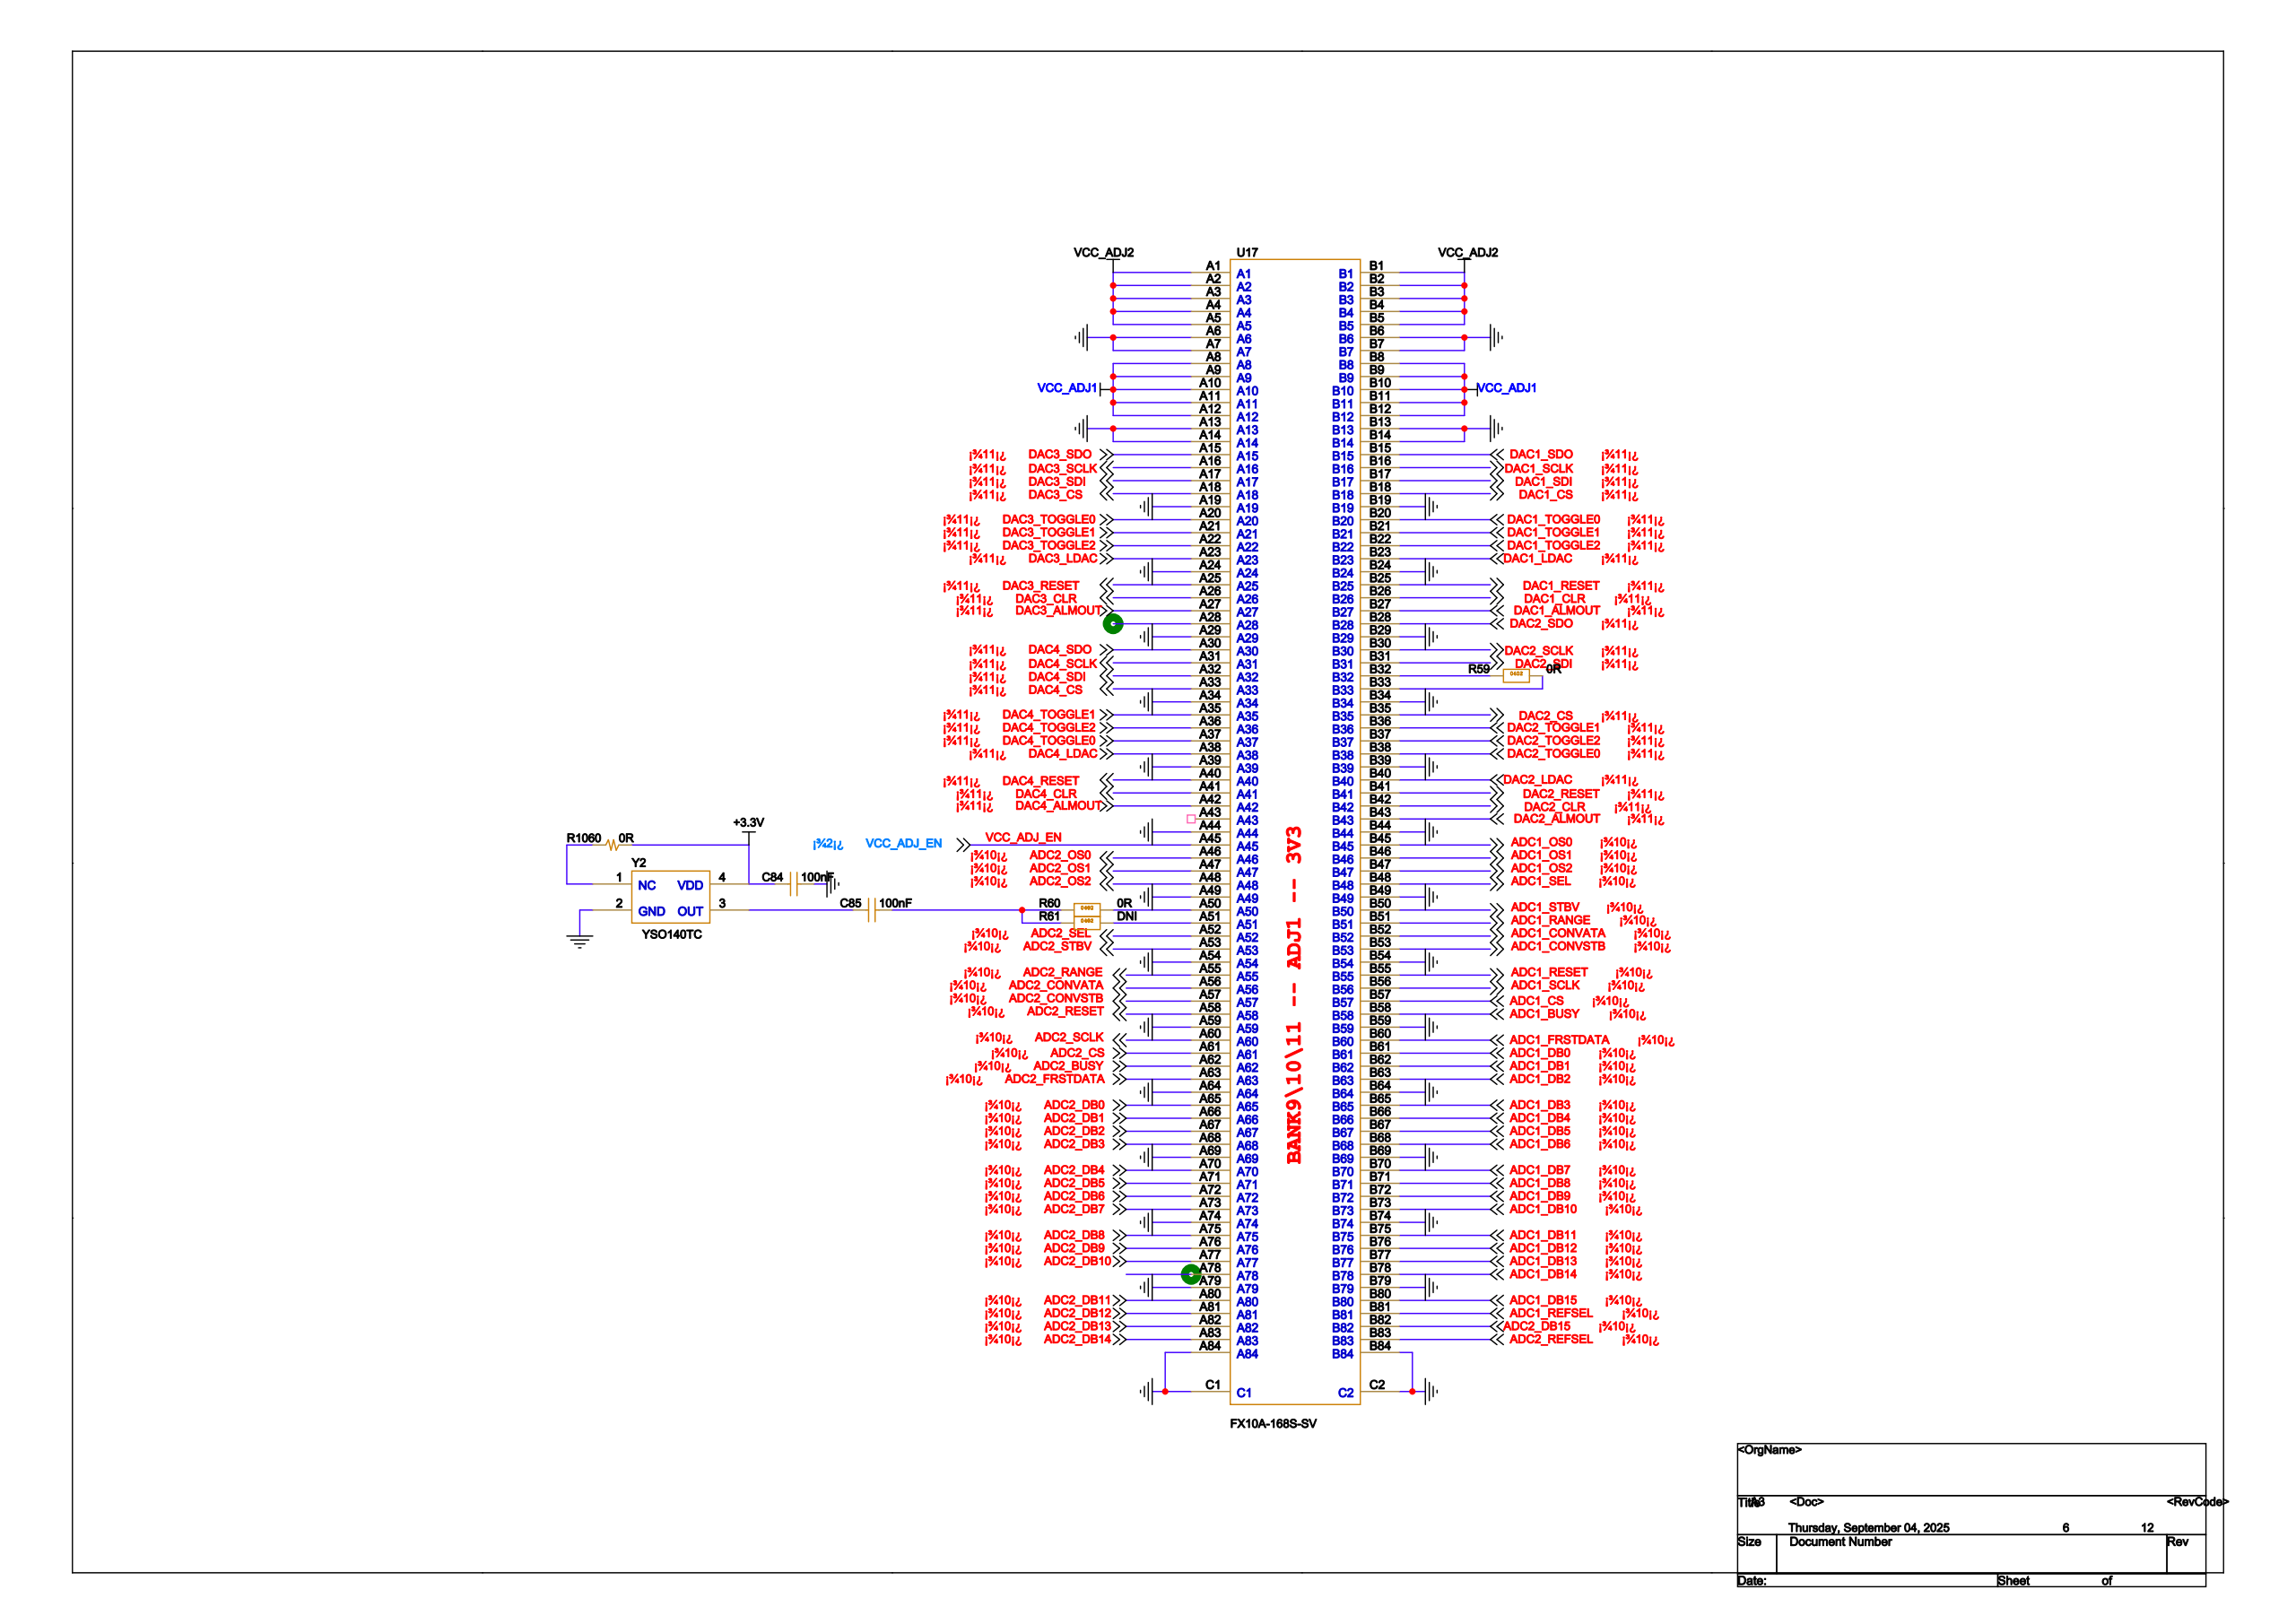Circuit board | Cadence Allegro | 528 parts | 530 nets | one sheet of the schematic
Parts on this sheet (reference | value | footprint):
C84 | 100nF | C0402
C85 | 100nF | C0402
R59 | 0R | R0402
R60 | 0R | R0402
R61 | DNI | R0402
R1060 | 0R | R0402
U17 | FX10A-168S-SV | FX10A-168S-SV
Y2 | YSO140TC | 3225-4
Nets of these parts (net: part-pin ...):
GND: C84-2 Y2-2 U17-A6 U17-A7 U17-A13 U17-A14 U17-A19 U17-A24 U17-A29 U17-A34 U17-A39 U17-A44 U17-A49 U17-A54 U17-A59 U17-A64 U17-A69 U17-A74 U17-A79 U17-A84 U17-B6 U17-B7 U17-B13 U17-B14 U17-B19 U17-B24 U17-B29 U17-B34 U17-B39 U17-B44 U17-B49 U17-B54 U17-B59 U17-B64 U17-B69 U17-B74 U17-B79 U17-B84 U17-C1 U17-C2
ADC1_BUSY: U17-B58
ADC1_CONVATA: U17-B52
ADC1_CONVSTB: U17-B53
ADC1_DB0: U17-B61
ADC1_DB10: U17-B73
ADC1_DB11: U17-B75
ADC1_DB12: U17-B76
ADC1_DB13: U17-B77
ADC1_DB14: U17-B78
ADC1_DB15: U17-B80
ADC1_DB1: U17-B62
ADC1_DB2: U17-B63
ADC1_DB3: U17-B65
ADC1_DB4: U17-B66
ADC1_DB5: U17-B67
ADC1_DB6: U17-B68
ADC1_DB7: U17-B70
ADC1_DB8: U17-B71
ADC1_DB9: U17-B72
ADC1_FRSTDATA: U17-B60
ADC1_OS0: U17-B45
ADC1_OS1: U17-B46
ADC1_OS2: U17-B47
ADC1_RANGE: U17-B51
ADC1_REFSEL: U17-B81
ADC1_RESET: U17-B55
ADC1_CS: U17-B57
ADC1_SEL: U17-B48
ADC1_SCLK: U17-B56
ADC1_STBV: U17-B50
ADC2_BUSY: U17-A62
ADC2_CONVATA: U17-A56
ADC2_CONVSTB: U17-A57
ADC2_DB0: U17-A65
ADC2_DB10: U17-A77
ADC2_DB11: U17-A80
ADC2_DB12: U17-A81
ADC2_DB13: U17-A82
ADC2_DB14: U17-A83
ADC2_DB15: U17-B82
ADC2_DB1: U17-A66
ADC2_DB2: U17-A67
ADC2_DB3: U17-A68
ADC2_DB4: U17-A70
ADC2_DB5: U17-A71
ADC2_DB6: U17-A72
ADC2_DB7: U17-A73
ADC2_DB8: U17-A75
ADC2_DB9: U17-A76
ADC2_FRSTDATA: U17-A63
ADC2_OS0: U17-A46
ADC2_OS1: U17-A47
ADC2_OS2: U17-A48
ADC2_RANGE: U17-A55
ADC2_REFSEL: U17-B83
ADC2_RESET: U17-A58
ADC2_CS: U17-A61
ADC2_SEL: U17-A52
ADC2_SCLK: U17-A60
ADC2_STBV: U17-A53
+3.3V: C84-1 R1060-2 Y2-4
N18886373: R1060-1 Y2-1
N18880414: C85-1 Y2-3
N18695571: C85-2 R60-1 R61-1
VCC_ADJ1: U17-A8 U17-A9 U17-A10 U17-A11 U17-A12 U17-B8 U17-B9 U17-B10 U17-B11 U17-B12
VCC_ADJ2: U17-A1 U17-A2 U17-A3 U17-A4 U17-A5 U17-B1 U17-B2 U17-B3 U17-B4 U17-B5
DAC1_ALMOUT: U17-B27
DAC2_ALMOUT: U17-B43
DAC3_ALMOUT: U17-A27
DAC4_ALMOUT: U17-A42
VCC_ADJ_EN: U17-A45
N18528843: R59-1 U17-B32
N18528846: R59-2 U17-B33
N18528610: R60-2 U17-A50
N18428157: R61-2 U17-A51
DAC3_SDO: U17-A15
DAC3_SCLK: U17-A16
DAC3_SDI: U17-A17
DAC3_CS: U17-A18
DAC3_TOGGLE0: U17-A20
DAC3_TOGGLE1: U17-A21
DAC3_TOGGLE2: U17-A22
DAC3_LDAC: U17-A23
DAC3_RESET: U17-A25
DAC3_CLR: U17-A26
DAC4_SDO: U17-A30
DAC4_SCLK: U17-A31
DAC4_SDI: U17-A32
DAC4_CS: U17-A33
DAC4_TOGGLE1: U17-A35
DAC4_TOGGLE2: U17-A36
DAC4_TOGGLE0: U17-A37
DAC4_LDAC: U17-A38
DAC4_RESET: U17-A40
DAC4_CLR: U17-A41
DAC1_SDO: U17-B15
DAC1_SCLK: U17-B16
DAC1_SDI: U17-B17
DAC1_CS: U17-B18
DAC1_TOGGLE0: U17-B20
DAC1_TOGGLE1: U17-B21
DAC1_TOGGLE2: U17-B22
DAC1_LDAC: U17-B23
DAC1_RESET: U17-B25
DAC1_CLR: U17-B26
DAC2_SDO: U17-B28
DAC2_SCLK: U17-B30
DAC2_SDI: U17-B31
DAC2_CS: U17-B35
DAC2_TOGGLE1: U17-B36
DAC2_TOGGLE2: U17-B37
DAC2_TOGGLE0: U17-B38
DAC2_LDAC: U17-B40
DAC2_RESET: U17-B41
DAC2_CLR: U17-B42